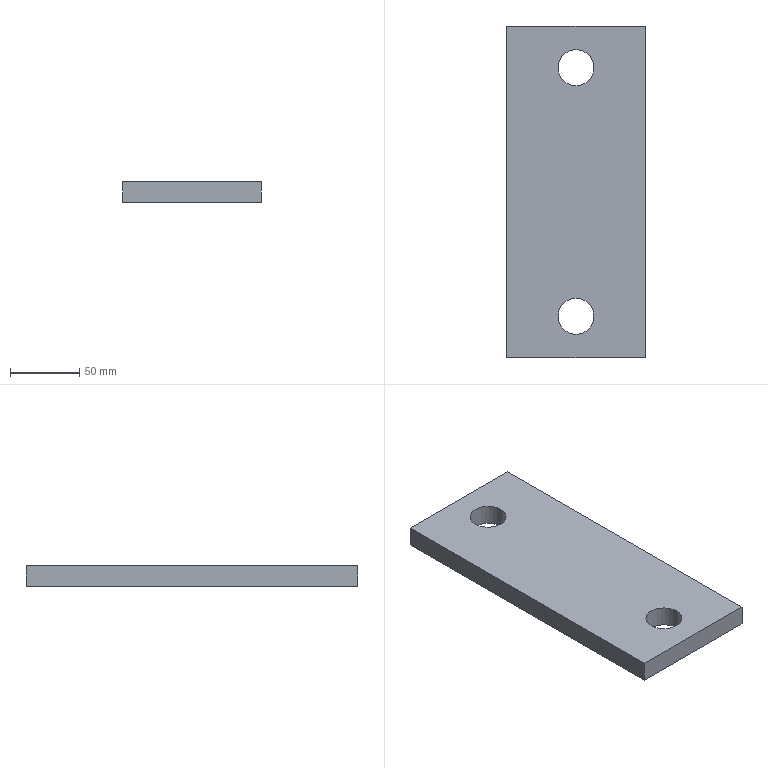Part | SolidWorks | features Extrusion 1, ICE 1 | 1 solid | 10 faces | box 100 x 240 x 15 mm | volume 344072 mm3 | plane 6 | cylinder 4 | commonest cylinder face diameters 26 x4
STEP:
#1=CARTESIAN_POINT('',(-13.,-90.,-7.5));
#2=VERTEX_POINT('',#1);
#3=CARTESIAN_POINT('',(13.,-90.,-7.5));
#4=VERTEX_POINT('',#3);
#5=CARTESIAN_POINT('',(0.,-90.,-7.5));
#6=DIRECTION('',(0.,0.,1.));
#7=DIRECTION('',(1.,0.,0.));
#8=AXIS2_PLACEMENT_3D('',#5,#6,#7);
#9=CIRCLE('',#8,13.);
#10=EDGE_CURVE('',#2,#4,#9,.T.);
#11=ORIENTED_EDGE('',*,*,#10,.F.);
#12=CARTESIAN_POINT('',(-13.,-90.,7.5));
#13=VERTEX_POINT('',#12);
#14=CARTESIAN_POINT('',(-13.,-90.,-24.5));
#15=DIRECTION('',(0.,0.,1.));
#16=VECTOR('',#15,1000.);
#17=LINE('',#14,#16);
#18=EDGE_CURVE('',#2,#13,#17,.T.);
#19=ORIENTED_EDGE('',*,*,#18,.T.);
#20=CARTESIAN_POINT('',(13.,-90.,7.5));
#21=VERTEX_POINT('',#20);
#22=CARTESIAN_POINT('',(0.,-90.,7.5));
#23=DIRECTION('',(0.,0.,1.));
#24=DIRECTION('',(1.,0.,0.));
#25=AXIS2_PLACEMENT_3D('',#22,#23,#24);
#26=CIRCLE('',#25,13.);
#27=EDGE_CURVE('',#13,#21,#26,.T.);
#28=ORIENTED_EDGE('',*,*,#27,.T.);
#29=CARTESIAN_POINT('',(13.,-90.,-24.5));
#30=DIRECTION('',(0.,0.,1.));
#31=VECTOR('',#30,1000.);
#32=LINE('',#29,#31);
#33=EDGE_CURVE('',#4,#21,#32,.T.);
#34=ORIENTED_EDGE('',*,*,#33,.F.);
#35=EDGE_LOOP('',(#11,#19,#28,#34));
#36=FACE_OUTER_BOUND('',#35,.T.);
#37=CARTESIAN_POINT('',(0.,-90.,-24.5));
#38=DIRECTION('',(0.,0.,1.));
#39=DIRECTION('',(1.,0.,0.));
#40=AXIS2_PLACEMENT_3D('',#37,#38,#39);
#41=CYLINDRICAL_SURFACE('',#40,13.);
#42=ADVANCED_FACE('',(#36),#41,.F.);
#43=CARTESIAN_POINT('',(-13.,90.,-7.5));
#44=VERTEX_POINT('',#43);
#45=CARTESIAN_POINT('',(13.,90.,-7.5));
#46=VERTEX_POINT('',#45);
#47=CARTESIAN_POINT('',(0.,90.,-7.5));
#48=DIRECTION('',(0.,0.,1.));
#49=DIRECTION('',(1.,0.,0.));
#50=AXIS2_PLACEMENT_3D('',#47,#48,#49);
#51=CIRCLE('',#50,13.);
#52=EDGE_CURVE('',#44,#46,#51,.T.);
#53=ORIENTED_EDGE('',*,*,#52,.F.);
#54=CARTESIAN_POINT('',(-13.,90.,7.5));
#55=VERTEX_POINT('',#54);
#56=CARTESIAN_POINT('',(-13.,90.,-24.5));
#57=DIRECTION('',(0.,0.,1.));
#58=VECTOR('',#57,1000.);
#59=LINE('',#56,#58);
#60=EDGE_CURVE('',#44,#55,#59,.T.);
#61=ORIENTED_EDGE('',*,*,#60,.T.);
#62=CARTESIAN_POINT('',(13.,90.,7.5));
#63=VERTEX_POINT('',#62);
#64=CARTESIAN_POINT('',(0.,90.,7.5));
#65=DIRECTION('',(0.,0.,1.));
#66=DIRECTION('',(1.,0.,0.));
#67=AXIS2_PLACEMENT_3D('',#64,#65,#66);
#68=CIRCLE('',#67,13.);
#69=EDGE_CURVE('',#55,#63,#68,.T.);
#70=ORIENTED_EDGE('',*,*,#69,.T.);
#71=CARTESIAN_POINT('',(13.,90.,-24.5));
#72=DIRECTION('',(0.,0.,1.));
#73=VECTOR('',#72,1000.);
#74=LINE('',#71,#73);
#75=EDGE_CURVE('',#46,#63,#74,.T.);
#76=ORIENTED_EDGE('',*,*,#75,.F.);
#77=EDGE_LOOP('',(#53,#61,#70,#76));
#78=FACE_OUTER_BOUND('',#77,.T.);
#79=CARTESIAN_POINT('',(0.,90.,-24.5));
#80=DIRECTION('',(0.,0.,1.));
#81=DIRECTION('',(1.,0.,0.));
#82=AXIS2_PLACEMENT_3D('',#79,#80,#81);
#83=CYLINDRICAL_SURFACE('',#82,13.);
#84=ADVANCED_FACE('',(#78),#83,.F.);
#85=CARTESIAN_POINT('',(-50.,120.,-7.5));
#86=VERTEX_POINT('',#85);
#87=CARTESIAN_POINT('',(-50.,-120.,-7.5));
#88=VERTEX_POINT('',#87);
#89=CARTESIAN_POINT('',(-50.,-120.,-7.5));
#90=DIRECTION('',(0.,-1.,0.));
#91=VECTOR('',#90,1000.);
#92=LINE('',#89,#91);
#93=EDGE_CURVE('',#86,#88,#92,.T.);
#94=ORIENTED_EDGE('',*,*,#93,.T.);
#95=CARTESIAN_POINT('',(-50.,-120.,7.5));
#96=VERTEX_POINT('',#95);
#97=CARTESIAN_POINT('',(-50.,-120.,7.5));
#98=DIRECTION('',(0.,0.,-1.));
#99=VECTOR('',#98,1000.);
#100=LINE('',#97,#99);
#101=EDGE_CURVE('',#96,#88,#100,.T.);
#102=ORIENTED_EDGE('',*,*,#101,.F.);
#103=CARTESIAN_POINT('',(-50.,120.,7.5));
#104=VERTEX_POINT('',#103);
#105=CARTESIAN_POINT('',(-50.,-120.,7.5));
#106=DIRECTION('',(0.,-1.,0.));
#107=VECTOR('',#106,1000.);
#108=LINE('',#105,#107);
#109=EDGE_CURVE('',#104,#96,#108,.T.);
#110=ORIENTED_EDGE('',*,*,#109,.F.);
#111=CARTESIAN_POINT('',(-50.,120.,7.5));
#112=DIRECTION('',(0.,0.,-1.));
#113=VECTOR('',#112,1000.);
#114=LINE('',#111,#113);
#115=EDGE_CURVE('',#104,#86,#114,.T.);
#116=ORIENTED_EDGE('',*,*,#115,.T.);
#117=EDGE_LOOP('',(#94,#102,#110,#116));
#118=FACE_OUTER_BOUND('',#117,.T.);
#119=CARTESIAN_POINT('',(-50.,-120.,7.5));
#120=DIRECTION('',(1.,0.,0.));
#121=DIRECTION('',(0.,0.,-1.));
#122=AXIS2_PLACEMENT_3D('',#119,#120,#121);
#123=PLANE('',#122);
#124=ADVANCED_FACE('',(#118),#123,.F.);
#125=CARTESIAN_POINT('',(50.,-120.,-7.5));
#126=VERTEX_POINT('',#125);
#127=CARTESIAN_POINT('',(50.,-120.,-7.5));
#128=DIRECTION('',(1.,0.,0.));
#129=VECTOR('',#128,1000.);
#130=LINE('',#127,#129);
#131=EDGE_CURVE('',#88,#126,#130,.T.);
#132=ORIENTED_EDGE('',*,*,#131,.T.);
#133=CARTESIAN_POINT('',(50.,-120.,7.5));
#134=VERTEX_POINT('',#133);
#135=CARTESIAN_POINT('',(50.,-120.,7.5));
#136=DIRECTION('',(0.,0.,-1.));
#137=VECTOR('',#136,1000.);
#138=LINE('',#135,#137);
#139=EDGE_CURVE('',#134,#126,#138,.T.);
#140=ORIENTED_EDGE('',*,*,#139,.F.);
#141=CARTESIAN_POINT('',(50.,-120.,7.5));
#142=DIRECTION('',(1.,0.,0.));
#143=VECTOR('',#142,1000.);
#144=LINE('',#141,#143);
#145=EDGE_CURVE('',#96,#134,#144,.T.);
#146=ORIENTED_EDGE('',*,*,#145,.F.);
#147=ORIENTED_EDGE('',*,*,#101,.T.);
#148=EDGE_LOOP('',(#132,#140,#146,#147));
#149=FACE_OUTER_BOUND('',#148,.T.);
#150=CARTESIAN_POINT('',(50.,-120.,7.5));
#151=DIRECTION('',(0.,1.,0.));
#152=DIRECTION('',(-1.,0.,0.));
#153=AXIS2_PLACEMENT_3D('',#150,#151,#152);
#154=PLANE('',#153);
#155=ADVANCED_FACE('',(#149),#154,.F.);
#156=CARTESIAN_POINT('',(50.,120.,-7.5));
#157=VERTEX_POINT('',#156);
#158=CARTESIAN_POINT('',(50.,-120.,-7.5));
#159=DIRECTION('',(0.,1.,0.));
#160=VECTOR('',#159,1000.);
#161=LINE('',#158,#160);
#162=EDGE_CURVE('',#126,#157,#161,.T.);
#163=ORIENTED_EDGE('',*,*,#162,.T.);
#164=CARTESIAN_POINT('',(50.,120.,7.5));
#165=VERTEX_POINT('',#164);
#166=CARTESIAN_POINT('',(50.,120.,7.5));
#167=DIRECTION('',(0.,0.,-1.));
#168=VECTOR('',#167,1000.);
#169=LINE('',#166,#168);
#170=EDGE_CURVE('',#165,#157,#169,.T.);
#171=ORIENTED_EDGE('',*,*,#170,.F.);
#172=CARTESIAN_POINT('',(50.,-120.,7.5));
#173=DIRECTION('',(0.,1.,0.));
#174=VECTOR('',#173,1000.);
#175=LINE('',#172,#174);
#176=EDGE_CURVE('',#134,#165,#175,.T.);
#177=ORIENTED_EDGE('',*,*,#176,.F.);
#178=ORIENTED_EDGE('',*,*,#139,.T.);
#179=EDGE_LOOP('',(#163,#171,#177,#178));
#180=FACE_OUTER_BOUND('',#179,.T.);
#181=CARTESIAN_POINT('',(50.,-120.,7.5));
#182=DIRECTION('',(-1.,0.,0.));
#183=DIRECTION('',(0.,0.,1.));
#184=AXIS2_PLACEMENT_3D('',#181,#182,#183);
#185=PLANE('',#184);
#186=ADVANCED_FACE('',(#180),#185,.F.);
#187=CARTESIAN_POINT('',(50.,120.,-7.5));
#188=DIRECTION('',(-1.,0.,0.));
#189=VECTOR('',#188,1000.);
#190=LINE('',#187,#189);
#191=EDGE_CURVE('',#157,#86,#190,.T.);
#192=ORIENTED_EDGE('',*,*,#191,.T.);
#193=ORIENTED_EDGE('',*,*,#115,.F.);
#194=CARTESIAN_POINT('',(50.,120.,7.5));
#195=DIRECTION('',(-1.,0.,0.));
#196=VECTOR('',#195,1000.);
#197=LINE('',#194,#196);
#198=EDGE_CURVE('',#165,#104,#197,.T.);
#199=ORIENTED_EDGE('',*,*,#198,.F.);
#200=ORIENTED_EDGE('',*,*,#170,.T.);
#201=EDGE_LOOP('',(#192,#193,#199,#200));
#202=FACE_OUTER_BOUND('',#201,.T.);
#203=CARTESIAN_POINT('',(50.,120.,7.5));
#204=DIRECTION('',(0.,-1.,0.));
#205=DIRECTION('',(1.,0.,0.));
#206=AXIS2_PLACEMENT_3D('',#203,#204,#205);
#207=PLANE('',#206);
#208=ADVANCED_FACE('',(#202),#207,.F.);
#209=CARTESIAN_POINT('',(0.,-90.,7.5));
#210=DIRECTION('',(0.,0.,1.));
#211=DIRECTION('',(1.,0.,0.));
#212=AXIS2_PLACEMENT_3D('',#209,#210,#211);
#213=CIRCLE('',#212,13.);
#214=EDGE_CURVE('',#21,#13,#213,.T.);
#215=ORIENTED_EDGE('',*,*,#214,.F.);
#216=ORIENTED_EDGE('',*,*,#27,.F.);
#217=EDGE_LOOP('',(#215,#216));
#218=FACE_BOUND('',#217,.T.);
#219=CARTESIAN_POINT('',(0.,90.,7.5));
#220=DIRECTION('',(0.,0.,1.));
#221=DIRECTION('',(1.,0.,0.));
#222=AXIS2_PLACEMENT_3D('',#219,#220,#221);
#223=CIRCLE('',#222,13.);
#224=EDGE_CURVE('',#63,#55,#223,.T.);
#225=ORIENTED_EDGE('',*,*,#224,.F.);
#226=ORIENTED_EDGE('',*,*,#69,.F.);
#227=EDGE_LOOP('',(#225,#226));
#228=FACE_BOUND('',#227,.T.);
#229=ORIENTED_EDGE('',*,*,#109,.T.);
#230=ORIENTED_EDGE('',*,*,#145,.T.);
#231=ORIENTED_EDGE('',*,*,#176,.T.);
#232=ORIENTED_EDGE('',*,*,#198,.T.);
#233=EDGE_LOOP('',(#229,#230,#231,#232));
#234=FACE_OUTER_BOUND('',#233,.T.);
#235=CARTESIAN_POINT('',(0.,0.,7.5));
#236=DIRECTION('',(0.,0.,1.));
#237=DIRECTION('',(1.,0.,0.));
#238=AXIS2_PLACEMENT_3D('',#235,#236,#237);
#239=PLANE('',#238);
#240=ADVANCED_FACE('',(#218,#228,#234),#239,.T.);
#241=CARTESIAN_POINT('',(0.,-90.,-7.5));
#242=DIRECTION('',(0.,0.,1.));
#243=DIRECTION('',(1.,0.,0.));
#244=AXIS2_PLACEMENT_3D('',#241,#242,#243);
#245=CIRCLE('',#244,13.);
#246=EDGE_CURVE('',#4,#2,#245,.T.);
#247=ORIENTED_EDGE('',*,*,#246,.T.);
#248=ORIENTED_EDGE('',*,*,#10,.T.);
#249=EDGE_LOOP('',(#247,#248));
#250=FACE_BOUND('',#249,.T.);
#251=CARTESIAN_POINT('',(0.,90.,-7.5));
#252=DIRECTION('',(0.,0.,1.));
#253=DIRECTION('',(1.,0.,0.));
#254=AXIS2_PLACEMENT_3D('',#251,#252,#253);
#255=CIRCLE('',#254,13.);
#256=EDGE_CURVE('',#46,#44,#255,.T.);
#257=ORIENTED_EDGE('',*,*,#256,.T.);
#258=ORIENTED_EDGE('',*,*,#52,.T.);
#259=EDGE_LOOP('',(#257,#258));
#260=FACE_BOUND('',#259,.T.);
#261=ORIENTED_EDGE('',*,*,#93,.F.);
#262=ORIENTED_EDGE('',*,*,#191,.F.);
#263=ORIENTED_EDGE('',*,*,#162,.F.);
#264=ORIENTED_EDGE('',*,*,#131,.F.);
#265=EDGE_LOOP('',(#261,#262,#263,#264));
#266=FACE_OUTER_BOUND('',#265,.T.);
#267=CARTESIAN_POINT('',(0.,0.,-7.5));
#268=DIRECTION('',(0.,0.,1.));
#269=DIRECTION('',(1.,0.,0.));
#270=AXIS2_PLACEMENT_3D('',#267,#268,#269);
#271=PLANE('',#270);
#272=ADVANCED_FACE('',(#250,#260,#266),#271,.F.);
#273=ORIENTED_EDGE('',*,*,#60,.F.);
#274=ORIENTED_EDGE('',*,*,#256,.F.);
#275=ORIENTED_EDGE('',*,*,#75,.T.);
#276=ORIENTED_EDGE('',*,*,#224,.T.);
#277=EDGE_LOOP('',(#273,#274,#275,#276));
#278=FACE_OUTER_BOUND('',#277,.T.);
#279=CARTESIAN_POINT('',(0.,90.,-24.5));
#280=DIRECTION('',(0.,0.,1.));
#281=DIRECTION('',(1.,0.,0.));
#282=AXIS2_PLACEMENT_3D('',#279,#280,#281);
#283=CYLINDRICAL_SURFACE('',#282,13.);
#284=ADVANCED_FACE('',(#278),#283,.F.);
#285=ORIENTED_EDGE('',*,*,#18,.F.);
#286=ORIENTED_EDGE('',*,*,#246,.F.);
#287=ORIENTED_EDGE('',*,*,#33,.T.);
#288=ORIENTED_EDGE('',*,*,#214,.T.);
#289=EDGE_LOOP('',(#285,#286,#287,#288));
#290=FACE_OUTER_BOUND('',#289,.T.);
#291=CARTESIAN_POINT('',(0.,-90.,-24.5));
#292=DIRECTION('',(0.,0.,1.));
#293=DIRECTION('',(1.,0.,0.));
#294=AXIS2_PLACEMENT_3D('',#291,#292,#293);
#295=CYLINDRICAL_SURFACE('',#294,13.);
#296=ADVANCED_FACE('',(#290),#295,.F.);
#297=CLOSED_SHELL('',(#42,#84,#124,#155,#186,#208,#240,#272,#284,#296));
#298=MANIFOLD_SOLID_BREP('',#297);
#299=CARTESIAN_POINT('',(0.,0.,0.));
#300=DIRECTION('',(0.,0.,1.));
#301=DIRECTION('',(1.,0.,0.));
#302=AXIS2_PLACEMENT_3D('',#299,#300,#301);
#303=(LENGTH_UNIT()NAMED_UNIT(*)SI_UNIT(.MILLI.,.METRE.));
#304=UNCERTAINTY_MEASURE_WITH_UNIT(LENGTH_MEASURE(0.00001),#303,'','');
#305=(NAMED_UNIT(*)PLANE_ANGLE_UNIT()SI_UNIT($,.RADIAN.));
#306=(NAMED_UNIT(*)SI_UNIT($,.STERADIAN.)SOLID_ANGLE_UNIT());
#307=(GEOMETRIC_REPRESENTATION_CONTEXT(3)GLOBAL_UNCERTAINTY_ASSIGNED_CONTEXT((#304))GLOBAL_UNIT_ASSIGNED_CONTEXT((#303,#305,#306))REPRESENTATION_CONTEXT('',''));
#308=ADVANCED_BREP_SHAPE_REPRESENTATION('',(#298,#302),#307);